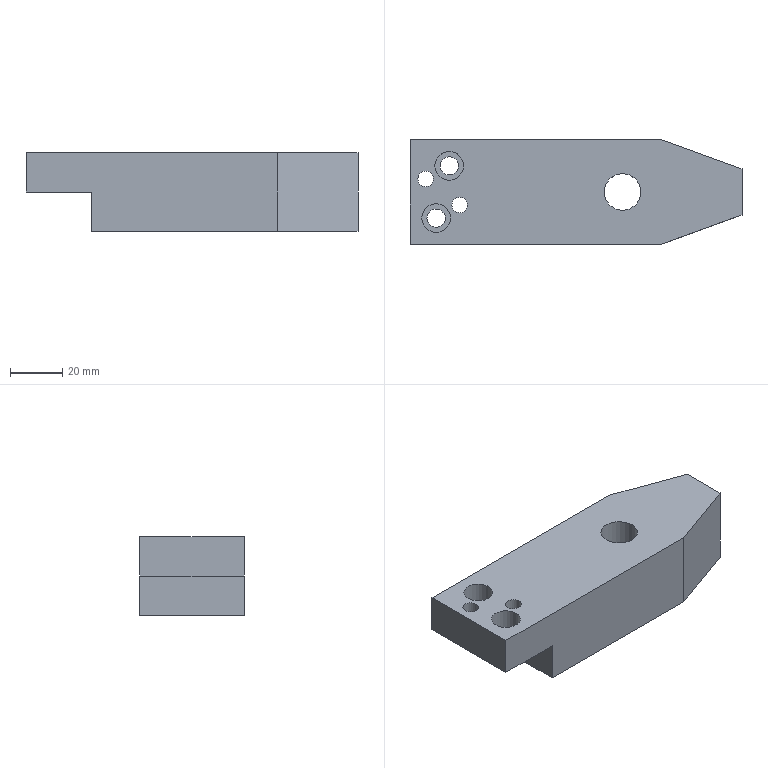Part | NX | features 22 2 | 1 solid | 19 faces | box 127 x 40 x 30 mm | volume 119314 mm3 | plane 12 | cylinder 7 | commonest cylinder face diameters 6.001 x2 7 x2 11 x2 14 x1
STEP:
#1=CARTESIAN_POINT('',(905.,-20.,-33.5));
#2=VERTEX_POINT('',#1);
#3=CARTESIAN_POINT('',(905.,20.,-33.5));
#4=VERTEX_POINT('',#3);
#5=CARTESIAN_POINT('',(905.,0.,-33.5));
#6=DIRECTION('',(0.,1.,0.));
#7=VECTOR('',#6,1000.);
#8=LINE('',#5,#7);
#9=EDGE_CURVE('',#2,#4,#8,.T.);
#10=ORIENTED_EDGE('',*,*,#9,.T.);
#11=CARTESIAN_POINT('',(976.236,20.,-33.5));
#12=VERTEX_POINT('',#11);
#13=CARTESIAN_POINT('',(908.,20.,-33.5));
#14=DIRECTION('',(-1.,0.,0.));
#15=VECTOR('',#14,1000.);
#16=LINE('',#13,#15);
#17=EDGE_CURVE('',#12,#4,#16,.T.);
#18=ORIENTED_EDGE('',*,*,#17,.F.);
#19=CARTESIAN_POINT('',(1007.,8.803,-33.5));
#20=VERTEX_POINT('',#19);
#21=CARTESIAN_POINT('',(922.41,39.591,-33.5));
#22=DIRECTION('',(0.9397,-0.342,0.));
#23=VECTOR('',#22,1000.);
#24=LINE('',#21,#23);
#25=EDGE_CURVE('',#12,#20,#24,.T.);
#26=ORIENTED_EDGE('',*,*,#25,.T.);
#27=CARTESIAN_POINT('',(1007.,-8.803,-33.5));
#28=VERTEX_POINT('',#27);
#29=CARTESIAN_POINT('',(1007.,0.,-33.5));
#30=DIRECTION('',(0.,1.,0.));
#31=VECTOR('',#30,1000.);
#32=LINE('',#29,#31);
#33=EDGE_CURVE('',#28,#20,#32,.T.);
#34=ORIENTED_EDGE('',*,*,#33,.F.);
#35=CARTESIAN_POINT('',(976.236,-20.,-33.5));
#36=VERTEX_POINT('',#35);
#37=CARTESIAN_POINT('',(922.41,-39.591,-33.5));
#38=DIRECTION('',(-0.9397,-0.342,0.));
#39=VECTOR('',#38,1000.);
#40=LINE('',#37,#39);
#41=EDGE_CURVE('',#28,#36,#40,.T.);
#42=ORIENTED_EDGE('',*,*,#41,.T.);
#43=CARTESIAN_POINT('',(908.,-20.,-33.5));
#44=DIRECTION('',(1.,0.,0.));
#45=VECTOR('',#44,1000.);
#46=LINE('',#43,#45);
#47=EDGE_CURVE('',#2,#36,#46,.T.);
#48=ORIENTED_EDGE('',*,*,#47,.F.);
#49=EDGE_LOOP('',(#10,#18,#26,#34,#42,#48));
#50=FACE_BOUND('',#49,.T.);
#51=CARTESIAN_POINT('',(954.306,0.,-33.5));
#52=VERTEX_POINT('',#51);
#53=CARTESIAN_POINT('',(961.306,0.,-33.5));
#54=DIRECTION('',(0.,0.,-1.));
#55=DIRECTION('',(-1.,0.,0.));
#56=AXIS2_PLACEMENT_3D('',#53,#54,#55);
#57=CIRCLE('',#56,7.);
#58=EDGE_CURVE('',#52,#52,#57,.T.);
#59=ORIENTED_EDGE('',*,*,#58,.F.);
#60=EDGE_LOOP('',(#59));
#61=FACE_BOUND('',#60,.T.);
#62=CARTESIAN_POINT('',(908.,0.,-33.5));
#63=DIRECTION('',(0.,0.,-1.));
#64=DIRECTION('',(1.,0.,0.));
#65=AXIS2_PLACEMENT_3D('',#62,#63,#64);
#66=PLANE('',#65);
#67=ADVANCED_FACE('',(#50,#61),#66,.T.);
#68=CARTESIAN_POINT('',(968.306,0.,-3.5));
#69=VERTEX_POINT('',#68);
#70=CARTESIAN_POINT('',(961.306,0.,-3.5));
#71=DIRECTION('',(0.,0.,1.));
#72=DIRECTION('',(1.,0.,0.));
#73=AXIS2_PLACEMENT_3D('',#70,#71,#72);
#74=CIRCLE('',#73,7.);
#75=EDGE_CURVE('',#69,#69,#74,.T.);
#76=ORIENTED_EDGE('',*,*,#75,.F.);
#77=EDGE_LOOP('',(#76));
#78=FACE_BOUND('',#77,.T.);
#79=CARTESIAN_POINT('',(889.5,10.,-3.5));
#80=VERTEX_POINT('',#79);
#81=CARTESIAN_POINT('',(895.,10.,-3.5));
#82=DIRECTION('',(0.,0.,1.));
#83=DIRECTION('',(-1.,0.,0.));
#84=AXIS2_PLACEMENT_3D('',#81,#82,#83);
#85=CIRCLE('',#84,5.5);
#86=EDGE_CURVE('',#80,#80,#85,.T.);
#87=ORIENTED_EDGE('',*,*,#86,.F.);
#88=EDGE_LOOP('',(#87));
#89=FACE_BOUND('',#88,.T.);
#90=CARTESIAN_POINT('',(902.001,-5.,-3.5));
#91=VERTEX_POINT('',#90);
#92=CARTESIAN_POINT('',(899.,-5.,-3.5));
#93=DIRECTION('',(0.,0.,1.));
#94=DIRECTION('',(1.,0.,0.));
#95=AXIS2_PLACEMENT_3D('',#92,#93,#94);
#96=CIRCLE('',#95,3.001);
#97=EDGE_CURVE('',#91,#91,#96,.T.);
#98=ORIENTED_EDGE('',*,*,#97,.F.);
#99=EDGE_LOOP('',(#98));
#100=FACE_BOUND('',#99,.T.);
#101=CARTESIAN_POINT('',(889.,5.,-3.5));
#102=VERTEX_POINT('',#101);
#103=CARTESIAN_POINT('',(886.,5.,-3.5));
#104=DIRECTION('',(0.,0.,1.));
#105=DIRECTION('',(1.,0.,0.));
#106=AXIS2_PLACEMENT_3D('',#103,#104,#105);
#107=CIRCLE('',#106,3.001);
#108=EDGE_CURVE('',#102,#102,#107,.T.);
#109=ORIENTED_EDGE('',*,*,#108,.F.);
#110=EDGE_LOOP('',(#109));
#111=FACE_BOUND('',#110,.T.);
#112=CARTESIAN_POINT('',(880.,20.,-3.5));
#113=VERTEX_POINT('',#112);
#114=CARTESIAN_POINT('',(976.236,20.,-3.5));
#115=VERTEX_POINT('',#114);
#116=CARTESIAN_POINT('',(908.,20.,-3.5));
#117=DIRECTION('',(1.,0.,0.));
#118=VECTOR('',#117,1000.);
#119=LINE('',#116,#118);
#120=EDGE_CURVE('',#113,#115,#119,.T.);
#121=ORIENTED_EDGE('',*,*,#120,.F.);
#122=CARTESIAN_POINT('',(880.,-20.,-3.5));
#123=VERTEX_POINT('',#122);
#124=CARTESIAN_POINT('',(880.,0.,-3.5));
#125=DIRECTION('',(0.,1.,0.));
#126=VECTOR('',#125,1000.);
#127=LINE('',#124,#126);
#128=EDGE_CURVE('',#123,#113,#127,.T.);
#129=ORIENTED_EDGE('',*,*,#128,.F.);
#130=CARTESIAN_POINT('',(976.236,-20.,-3.5));
#131=VERTEX_POINT('',#130);
#132=CARTESIAN_POINT('',(908.,-20.,-3.5));
#133=DIRECTION('',(-1.,0.,0.));
#134=VECTOR('',#133,1000.);
#135=LINE('',#132,#134);
#136=EDGE_CURVE('',#131,#123,#135,.T.);
#137=ORIENTED_EDGE('',*,*,#136,.F.);
#138=CARTESIAN_POINT('',(1007.,-8.803,-3.5));
#139=VERTEX_POINT('',#138);
#140=CARTESIAN_POINT('',(922.41,-39.591,-3.5));
#141=DIRECTION('',(0.9397,0.342,0.));
#142=VECTOR('',#141,1000.);
#143=LINE('',#140,#142);
#144=EDGE_CURVE('',#131,#139,#143,.T.);
#145=ORIENTED_EDGE('',*,*,#144,.T.);
#146=CARTESIAN_POINT('',(1007.,8.803,-3.5));
#147=VERTEX_POINT('',#146);
#148=CARTESIAN_POINT('',(1007.,0.,-3.5));
#149=DIRECTION('',(0.,-1.,0.));
#150=VECTOR('',#149,1000.);
#151=LINE('',#148,#150);
#152=EDGE_CURVE('',#147,#139,#151,.T.);
#153=ORIENTED_EDGE('',*,*,#152,.F.);
#154=CARTESIAN_POINT('',(922.41,39.591,-3.5));
#155=DIRECTION('',(-0.9397,0.342,0.));
#156=VECTOR('',#155,1000.);
#157=LINE('',#154,#156);
#158=EDGE_CURVE('',#147,#115,#157,.T.);
#159=ORIENTED_EDGE('',*,*,#158,.T.);
#160=EDGE_LOOP('',(#121,#129,#137,#145,#153,#159));
#161=FACE_BOUND('',#160,.T.);
#162=CARTESIAN_POINT('',(895.5,-10.,-3.5));
#163=VERTEX_POINT('',#162);
#164=CARTESIAN_POINT('',(890.,-10.,-3.5));
#165=DIRECTION('',(0.,0.,-1.));
#166=DIRECTION('',(1.,0.,0.));
#167=AXIS2_PLACEMENT_3D('',#164,#165,#166);
#168=CIRCLE('',#167,5.5);
#169=EDGE_CURVE('',#163,#163,#168,.T.);
#170=ORIENTED_EDGE('',*,*,#169,.T.);
#171=EDGE_LOOP('',(#170));
#172=FACE_BOUND('',#171,.T.);
#173=CARTESIAN_POINT('',(908.,0.,-3.5));
#174=DIRECTION('',(0.,0.,1.));
#175=DIRECTION('',(-1.,0.,0.));
#176=AXIS2_PLACEMENT_3D('',#173,#174,#175);
#177=PLANE('',#176);
#178=ADVANCED_FACE('',(#78,#89,#100,#111,#161,#172),#177,.T.);
#179=CARTESIAN_POINT('',(905.,20.,-18.5));
#180=VERTEX_POINT('',#179);
#181=CARTESIAN_POINT('',(905.,-20.,-18.5));
#182=VERTEX_POINT('',#181);
#183=CARTESIAN_POINT('',(905.,0.,-18.5));
#184=DIRECTION('',(0.,-1.,0.));
#185=VECTOR('',#184,1000.);
#186=LINE('',#183,#185);
#187=EDGE_CURVE('',#180,#182,#186,.T.);
#188=ORIENTED_EDGE('',*,*,#187,.F.);
#189=CARTESIAN_POINT('',(905.,20.,-18.5));
#190=DIRECTION('',(0.,0.,-1.));
#191=VECTOR('',#190,1000.);
#192=LINE('',#189,#191);
#193=EDGE_CURVE('',#180,#4,#192,.T.);
#194=ORIENTED_EDGE('',*,*,#193,.T.);
#195=ORIENTED_EDGE('',*,*,#9,.F.);
#196=CARTESIAN_POINT('',(905.,-20.,-18.5));
#197=DIRECTION('',(0.,0.,1.));
#198=VECTOR('',#197,1000.);
#199=LINE('',#196,#198);
#200=EDGE_CURVE('',#2,#182,#199,.T.);
#201=ORIENTED_EDGE('',*,*,#200,.T.);
#202=EDGE_LOOP('',(#188,#194,#195,#201));
#203=FACE_BOUND('',#202,.T.);
#204=CARTESIAN_POINT('',(905.,0.,-21.));
#205=DIRECTION('',(1.,0.,0.));
#206=DIRECTION('',(0.,0.,1.));
#207=AXIS2_PLACEMENT_3D('',#204,#205,#206);
#208=PLANE('',#207);
#209=ADVANCED_FACE('',(#203),#208,.F.);
#210=ORIENTED_EDGE('',*,*,#144,.F.);
#211=CARTESIAN_POINT('',(976.236,-20.,-18.5));
#212=DIRECTION('',(0.,0.,1.));
#213=VECTOR('',#212,1000.);
#214=LINE('',#211,#213);
#215=EDGE_CURVE('',#36,#131,#214,.T.);
#216=ORIENTED_EDGE('',*,*,#215,.F.);
#217=ORIENTED_EDGE('',*,*,#41,.F.);
#218=CARTESIAN_POINT('',(1007.,-8.803,-18.5));
#219=DIRECTION('',(0.,0.,-1.));
#220=VECTOR('',#219,1000.);
#221=LINE('',#218,#220);
#222=EDGE_CURVE('',#139,#28,#221,.T.);
#223=ORIENTED_EDGE('',*,*,#222,.F.);
#224=EDGE_LOOP('',(#210,#216,#217,#223));
#225=FACE_BOUND('',#224,.T.);
#226=CARTESIAN_POINT('',(1012.547,-6.784,-13.5));
#227=DIRECTION('',(0.342,-0.9397,0.));
#228=DIRECTION('',(0.9397,0.342,0.));
#229=AXIS2_PLACEMENT_3D('',#226,#227,#228);
#230=PLANE('',#229);
#231=ADVANCED_FACE('',(#225),#230,.T.);
#232=ORIENTED_EDGE('',*,*,#193,.F.);
#233=CARTESIAN_POINT('',(880.,20.,-18.5));
#234=VERTEX_POINT('',#233);
#235=CARTESIAN_POINT('',(908.,20.,-18.5));
#236=DIRECTION('',(-1.,0.,0.));
#237=VECTOR('',#236,1000.);
#238=LINE('',#235,#237);
#239=EDGE_CURVE('',#180,#234,#238,.T.);
#240=ORIENTED_EDGE('',*,*,#239,.T.);
#241=CARTESIAN_POINT('',(880.,20.,-18.5));
#242=DIRECTION('',(0.,0.,1.));
#243=VECTOR('',#242,1000.);
#244=LINE('',#241,#243);
#245=EDGE_CURVE('',#234,#113,#244,.T.);
#246=ORIENTED_EDGE('',*,*,#245,.T.);
#247=ORIENTED_EDGE('',*,*,#120,.T.);
#248=CARTESIAN_POINT('',(976.236,20.,-18.5));
#249=DIRECTION('',(0.,0.,-1.));
#250=VECTOR('',#249,1000.);
#251=LINE('',#248,#250);
#252=EDGE_CURVE('',#115,#12,#251,.T.);
#253=ORIENTED_EDGE('',*,*,#252,.T.);
#254=ORIENTED_EDGE('',*,*,#17,.T.);
#255=EDGE_LOOP('',(#232,#240,#246,#247,#253,#254));
#256=FACE_BOUND('',#255,.T.);
#257=CARTESIAN_POINT('',(908.,20.,-18.5));
#258=DIRECTION('',(0.,1.,0.));
#259=DIRECTION('',(0.,0.,-1.));
#260=AXIS2_PLACEMENT_3D('',#257,#258,#259);
#261=PLANE('',#260);
#262=ADVANCED_FACE('',(#256),#261,.T.);
#263=ORIENTED_EDGE('',*,*,#158,.F.);
#264=CARTESIAN_POINT('',(1007.,8.803,-18.5));
#265=DIRECTION('',(0.,0.,1.));
#266=VECTOR('',#265,1000.);
#267=LINE('',#264,#266);
#268=EDGE_CURVE('',#20,#147,#267,.T.);
#269=ORIENTED_EDGE('',*,*,#268,.F.);
#270=ORIENTED_EDGE('',*,*,#25,.F.);
#271=ORIENTED_EDGE('',*,*,#252,.F.);
#272=EDGE_LOOP('',(#263,#269,#270,#271));
#273=FACE_BOUND('',#272,.T.);
#274=CARTESIAN_POINT('',(1012.547,6.784,-13.5));
#275=DIRECTION('',(0.342,0.9397,0.));
#276=DIRECTION('',(0.9397,-0.342,0.));
#277=AXIS2_PLACEMENT_3D('',#274,#275,#276);
#278=PLANE('',#277);
#279=ADVANCED_FACE('',(#273),#278,.T.);
#280=ORIENTED_EDGE('',*,*,#200,.F.);
#281=ORIENTED_EDGE('',*,*,#47,.T.);
#282=ORIENTED_EDGE('',*,*,#215,.T.);
#283=ORIENTED_EDGE('',*,*,#136,.T.);
#284=CARTESIAN_POINT('',(880.,-20.,-18.5));
#285=VERTEX_POINT('',#284);
#286=CARTESIAN_POINT('',(880.,-20.,-18.5));
#287=DIRECTION('',(0.,0.,1.));
#288=VECTOR('',#287,1000.);
#289=LINE('',#286,#288);
#290=EDGE_CURVE('',#285,#123,#289,.T.);
#291=ORIENTED_EDGE('',*,*,#290,.F.);
#292=CARTESIAN_POINT('',(908.,-20.,-18.5));
#293=DIRECTION('',(1.,0.,0.));
#294=VECTOR('',#293,1000.);
#295=LINE('',#292,#294);
#296=EDGE_CURVE('',#285,#182,#295,.T.);
#297=ORIENTED_EDGE('',*,*,#296,.T.);
#298=EDGE_LOOP('',(#280,#281,#282,#283,#291,#297));
#299=FACE_BOUND('',#298,.T.);
#300=CARTESIAN_POINT('',(908.,-20.,-18.5));
#301=DIRECTION('',(0.,-1.,0.));
#302=DIRECTION('',(0.,0.,1.));
#303=AXIS2_PLACEMENT_3D('',#300,#301,#302);
#304=PLANE('',#303);
#305=ADVANCED_FACE('',(#299),#304,.T.);
#306=ORIENTED_EDGE('',*,*,#152,.T.);
#307=ORIENTED_EDGE('',*,*,#222,.T.);
#308=ORIENTED_EDGE('',*,*,#33,.T.);
#309=ORIENTED_EDGE('',*,*,#268,.T.);
#310=EDGE_LOOP('',(#306,#307,#308,#309));
#311=FACE_BOUND('',#310,.T.);
#312=CARTESIAN_POINT('',(1007.,0.,-18.5));
#313=DIRECTION('',(1.,0.,0.));
#314=DIRECTION('',(0.,0.,1.));
#315=AXIS2_PLACEMENT_3D('',#312,#313,#314);
#316=PLANE('',#315);
#317=ADVANCED_FACE('',(#311),#316,.T.);
#318=ORIENTED_EDGE('',*,*,#290,.T.);
#319=ORIENTED_EDGE('',*,*,#128,.T.);
#320=ORIENTED_EDGE('',*,*,#245,.F.);
#321=CARTESIAN_POINT('',(880.,0.,-18.5));
#322=DIRECTION('',(0.,-1.,0.));
#323=VECTOR('',#322,1000.);
#324=LINE('',#321,#323);
#325=EDGE_CURVE('',#234,#285,#324,.T.);
#326=ORIENTED_EDGE('',*,*,#325,.T.);
#327=EDGE_LOOP('',(#318,#319,#320,#326));
#328=FACE_BOUND('',#327,.T.);
#329=CARTESIAN_POINT('',(880.,0.,-18.5));
#330=DIRECTION('',(-1.,0.,0.));
#331=DIRECTION('',(0.,0.,-1.));
#332=AXIS2_PLACEMENT_3D('',#329,#330,#331);
#333=PLANE('',#332);
#334=ADVANCED_FACE('',(#328),#333,.T.);
#335=CARTESIAN_POINT('',(891.5,10.,-18.5));
#336=VERTEX_POINT('',#335);
#337=CARTESIAN_POINT('',(895.,10.,-18.5));
#338=DIRECTION('',(0.,0.,-1.));
#339=DIRECTION('',(-1.,0.,0.));
#340=AXIS2_PLACEMENT_3D('',#337,#338,#339);
#341=CIRCLE('',#340,3.5);
#342=EDGE_CURVE('',#336,#336,#341,.T.);
#343=ORIENTED_EDGE('',*,*,#342,.F.);
#344=EDGE_LOOP('',(#343));
#345=FACE_BOUND('',#344,.T.);
#346=CARTESIAN_POINT('',(896.,-5.,-18.5));
#347=VERTEX_POINT('',#346);
#348=CARTESIAN_POINT('',(899.,-5.,-18.5));
#349=DIRECTION('',(0.,0.,-1.));
#350=DIRECTION('',(-1.,0.,0.));
#351=AXIS2_PLACEMENT_3D('',#348,#349,#350);
#352=CIRCLE('',#351,3.001);
#353=EDGE_CURVE('',#347,#347,#352,.T.);
#354=ORIENTED_EDGE('',*,*,#353,.F.);
#355=EDGE_LOOP('',(#354));
#356=FACE_BOUND('',#355,.T.);
#357=CARTESIAN_POINT('',(882.999,5.,-18.5));
#358=VERTEX_POINT('',#357);
#359=CARTESIAN_POINT('',(886.,5.,-18.5));
#360=DIRECTION('',(0.,0.,-1.));
#361=DIRECTION('',(-1.,0.,0.));
#362=AXIS2_PLACEMENT_3D('',#359,#360,#361);
#363=CIRCLE('',#362,3.001);
#364=EDGE_CURVE('',#358,#358,#363,.T.);
#365=ORIENTED_EDGE('',*,*,#364,.F.);
#366=EDGE_LOOP('',(#365));
#367=FACE_BOUND('',#366,.T.);
#368=CARTESIAN_POINT('',(886.5,-10.,-18.5));
#369=VERTEX_POINT('',#368);
#370=CARTESIAN_POINT('',(890.,-10.,-18.5));
#371=DIRECTION('',(0.,0.,-1.));
#372=DIRECTION('',(-1.,0.,0.));
#373=AXIS2_PLACEMENT_3D('',#370,#371,#372);
#374=CIRCLE('',#373,3.5);
#375=EDGE_CURVE('',#369,#369,#374,.T.);
#376=ORIENTED_EDGE('',*,*,#375,.F.);
#377=EDGE_LOOP('',(#376));
#378=FACE_BOUND('',#377,.T.);
#379=ORIENTED_EDGE('',*,*,#239,.F.);
#380=ORIENTED_EDGE('',*,*,#187,.T.);
#381=ORIENTED_EDGE('',*,*,#296,.F.);
#382=ORIENTED_EDGE('',*,*,#325,.F.);
#383=EDGE_LOOP('',(#379,#380,#381,#382));
#384=FACE_BOUND('',#383,.T.);
#385=CARTESIAN_POINT('',(908.,0.,-18.5));
#386=DIRECTION('',(0.,0.,-1.));
#387=DIRECTION('',(1.,0.,0.));
#388=AXIS2_PLACEMENT_3D('',#385,#386,#387);
#389=PLANE('',#388);
#390=ADVANCED_FACE('',(#345,#356,#367,#378,#384),#389,.T.);
#391=ORIENTED_EDGE('',*,*,#375,.T.);
#392=EDGE_LOOP('',(#391));
#393=FACE_BOUND('',#392,.T.);
#394=CARTESIAN_POINT('',(886.5,-10.,-13.5));
#395=VERTEX_POINT('',#394);
#396=CARTESIAN_POINT('',(890.,-10.,-13.5));
#397=DIRECTION('',(0.,0.,-1.));
#398=DIRECTION('',(-1.,0.,0.));
#399=AXIS2_PLACEMENT_3D('',#396,#397,#398);
#400=CIRCLE('',#399,3.5);
#401=EDGE_CURVE('',#395,#395,#400,.T.);
#402=ORIENTED_EDGE('',*,*,#401,.F.);
#403=EDGE_LOOP('',(#402));
#404=FACE_BOUND('',#403,.T.);
#405=CARTESIAN_POINT('',(890.,-10.,-1.5));
#406=DIRECTION('',(0.,0.,-1.));
#407=DIRECTION('',(-1.,0.,0.));
#408=AXIS2_PLACEMENT_3D('',#405,#406,#407);
#409=CYLINDRICAL_SURFACE('',#408,3.5);
#410=ADVANCED_FACE('',(#393,#404),#409,.F.);
#411=ORIENTED_EDGE('',*,*,#401,.T.);
#412=EDGE_LOOP('',(#411));
#413=FACE_BOUND('',#412,.T.);
#414=CARTESIAN_POINT('',(895.5,-10.,-13.5));
#415=VERTEX_POINT('',#414);
#416=CARTESIAN_POINT('',(890.,-10.,-13.5));
#417=DIRECTION('',(0.,0.,-1.));
#418=DIRECTION('',(1.,0.,0.));
#419=AXIS2_PLACEMENT_3D('',#416,#417,#418);
#420=CIRCLE('',#419,5.5);
#421=EDGE_CURVE('',#415,#415,#420,.T.);
#422=ORIENTED_EDGE('',*,*,#421,.F.);
#423=EDGE_LOOP('',(#422));
#424=FACE_BOUND('',#423,.T.);
#425=CARTESIAN_POINT('',(890.,-10.,-13.5));
#426=DIRECTION('',(0.,0.,-1.));
#427=DIRECTION('',(1.,0.,0.));
#428=AXIS2_PLACEMENT_3D('',#425,#426,#427);
#429=PLANE('',#428);
#430=ADVANCED_FACE('',(#413,#424),#429,.F.);
#431=ORIENTED_EDGE('',*,*,#421,.T.);
#432=EDGE_LOOP('',(#431));
#433=FACE_BOUND('',#432,.T.);
#434=ORIENTED_EDGE('',*,*,#169,.F.);
#435=EDGE_LOOP('',(#434));
#436=FACE_BOUND('',#435,.T.);
#437=CARTESIAN_POINT('',(890.,-10.,-3.5));
#438=DIRECTION('',(0.,0.,-1.));
#439=DIRECTION('',(-1.,0.,0.));
#440=AXIS2_PLACEMENT_3D('',#437,#438,#439);
#441=CYLINDRICAL_SURFACE('',#440,5.5);
#442=ADVANCED_FACE('',(#433,#436),#441,.F.);
#443=ORIENTED_EDGE('',*,*,#108,.T.);
#444=EDGE_LOOP('',(#443));
#445=FACE_BOUND('',#444,.T.);
#446=ORIENTED_EDGE('',*,*,#364,.T.);
#447=EDGE_LOOP('',(#446));
#448=FACE_BOUND('',#447,.T.);
#449=CARTESIAN_POINT('',(886.,5.,-1.5));
#450=DIRECTION('',(0.,0.,-1.));
#451=DIRECTION('',(-1.,0.,0.));
#452=AXIS2_PLACEMENT_3D('',#449,#450,#451);
#453=CYLINDRICAL_SURFACE('',#452,3.001);
#454=ADVANCED_FACE('',(#445,#448),#453,.F.);
#455=ORIENTED_EDGE('',*,*,#97,.T.);
#456=EDGE_LOOP('',(#455));
#457=FACE_BOUND('',#456,.T.);
#458=ORIENTED_EDGE('',*,*,#353,.T.);
#459=EDGE_LOOP('',(#458));
#460=FACE_BOUND('',#459,.T.);
#461=CARTESIAN_POINT('',(899.,-5.,-1.5));
#462=DIRECTION('',(0.,0.,-1.));
#463=DIRECTION('',(1.,0.,0.));
#464=AXIS2_PLACEMENT_3D('',#461,#462,#463);
#465=CYLINDRICAL_SURFACE('',#464,3.001);
#466=ADVANCED_FACE('',(#457,#460),#465,.F.);
#467=ORIENTED_EDGE('',*,*,#342,.T.);
#468=EDGE_LOOP('',(#467));
#469=FACE_BOUND('',#468,.T.);
#470=CARTESIAN_POINT('',(898.5,10.,-13.5));
#471=VERTEX_POINT('',#470);
#472=CARTESIAN_POINT('',(895.,10.,-13.5));
#473=DIRECTION('',(0.,0.,1.));
#474=DIRECTION('',(1.,0.,0.));
#475=AXIS2_PLACEMENT_3D('',#472,#473,#474);
#476=CIRCLE('',#475,3.5);
#477=EDGE_CURVE('',#471,#471,#476,.T.);
#478=ORIENTED_EDGE('',*,*,#477,.T.);
#479=EDGE_LOOP('',(#478));
#480=FACE_BOUND('',#479,.T.);
#481=CARTESIAN_POINT('',(895.,10.,-1.5));
#482=DIRECTION('',(0.,0.,-1.));
#483=DIRECTION('',(1.,0.,0.));
#484=AXIS2_PLACEMENT_3D('',#481,#482,#483);
#485=CYLINDRICAL_SURFACE('',#484,3.5);
#486=ADVANCED_FACE('',(#469,#480),#485,.F.);
#487=ORIENTED_EDGE('',*,*,#477,.F.);
#488=EDGE_LOOP('',(#487));
#489=FACE_BOUND('',#488,.T.);
#490=CARTESIAN_POINT('',(889.5,10.,-13.5));
#491=VERTEX_POINT('',#490);
#492=CARTESIAN_POINT('',(895.,10.,-13.5));
#493=DIRECTION('',(0.,0.,1.));
#494=DIRECTION('',(-1.,0.,0.));
#495=AXIS2_PLACEMENT_3D('',#492,#493,#494);
#496=CIRCLE('',#495,5.5);
#497=EDGE_CURVE('',#491,#491,#496,.T.);
#498=ORIENTED_EDGE('',*,*,#497,.T.);
#499=EDGE_LOOP('',(#498));
#500=FACE_BOUND('',#499,.T.);
#501=CARTESIAN_POINT('',(895.,10.,-13.5));
#502=DIRECTION('',(0.,0.,-1.));
#503=DIRECTION('',(-1.,0.,0.));
#504=AXIS2_PLACEMENT_3D('',#501,#502,#503);
#505=PLANE('',#504);
#506=ADVANCED_FACE('',(#489,#500),#505,.F.);
#507=ORIENTED_EDGE('',*,*,#497,.F.);
#508=EDGE_LOOP('',(#507));
#509=FACE_BOUND('',#508,.T.);
#510=ORIENTED_EDGE('',*,*,#86,.T.);
#511=EDGE_LOOP('',(#510));
#512=FACE_BOUND('',#511,.T.);
#513=CARTESIAN_POINT('',(895.,10.,-3.5));
#514=DIRECTION('',(0.,0.,-1.));
#515=DIRECTION('',(1.,0.,0.));
#516=AXIS2_PLACEMENT_3D('',#513,#514,#515);
#517=CYLINDRICAL_SURFACE('',#516,5.5);
#518=ADVANCED_FACE('',(#509,#512),#517,.F.);
#519=ORIENTED_EDGE('',*,*,#75,.T.);
#520=EDGE_LOOP('',(#519));
#521=FACE_BOUND('',#520,.T.);
#522=ORIENTED_EDGE('',*,*,#58,.T.);
#523=EDGE_LOOP('',(#522));
#524=FACE_BOUND('',#523,.T.);
#525=CARTESIAN_POINT('',(961.306,0.,6.));
#526=DIRECTION('',(0.,0.,-1.));
#527=DIRECTION('',(-1.,0.,0.));
#528=AXIS2_PLACEMENT_3D('',#525,#526,#527);
#529=CYLINDRICAL_SURFACE('',#528,7.);
#530=ADVANCED_FACE('',(#521,#524),#529,.F.);
#531=CLOSED_SHELL('',(#67,#178,#209,#231,#262,#279,#305,#317,#334,#390,#410,#430,#442,#454,#466,#486,#506,#518,#530));
#532=MANIFOLD_SOLID_BREP('',#531);
#533=(LENGTH_UNIT()NAMED_UNIT(*)SI_UNIT(.MILLI.,.METRE.));
#534=UNCERTAINTY_MEASURE_WITH_UNIT(LENGTH_MEASURE(0.00001),#533,'','');
#535=(NAMED_UNIT(*)PLANE_ANGLE_UNIT()SI_UNIT($,.RADIAN.));
#536=(NAMED_UNIT(*)SI_UNIT($,.STERADIAN.)SOLID_ANGLE_UNIT());
#537=(GEOMETRIC_REPRESENTATION_CONTEXT(3)GLOBAL_UNCERTAINTY_ASSIGNED_CONTEXT((#534))GLOBAL_UNIT_ASSIGNED_CONTEXT((#533,#535,#536))REPRESENTATION_CONTEXT('',''));
#538=ADVANCED_BREP_SHAPE_REPRESENTATION('',(#532),#537);